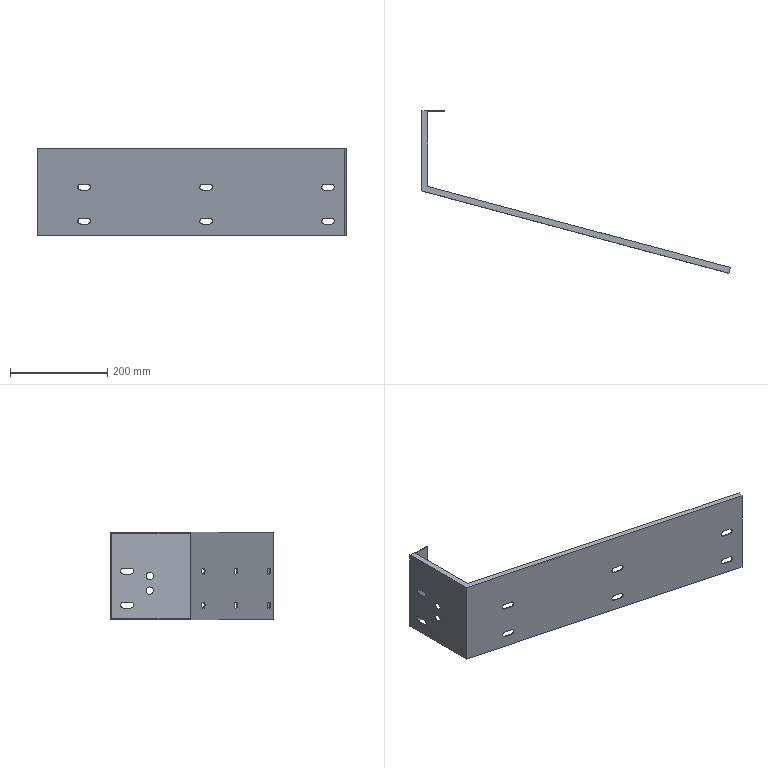Part | SolidWorks | features ICE 4, LPattern 3, BossThin 2, ExtruThin 1 | 1 solid | 60 faces | box 635.787 x 334.526 x 180 mm | volume 341333 mm3 | plane 34 | cylinder 26 | commonest cylinder face diameters 12 x22 15 x4